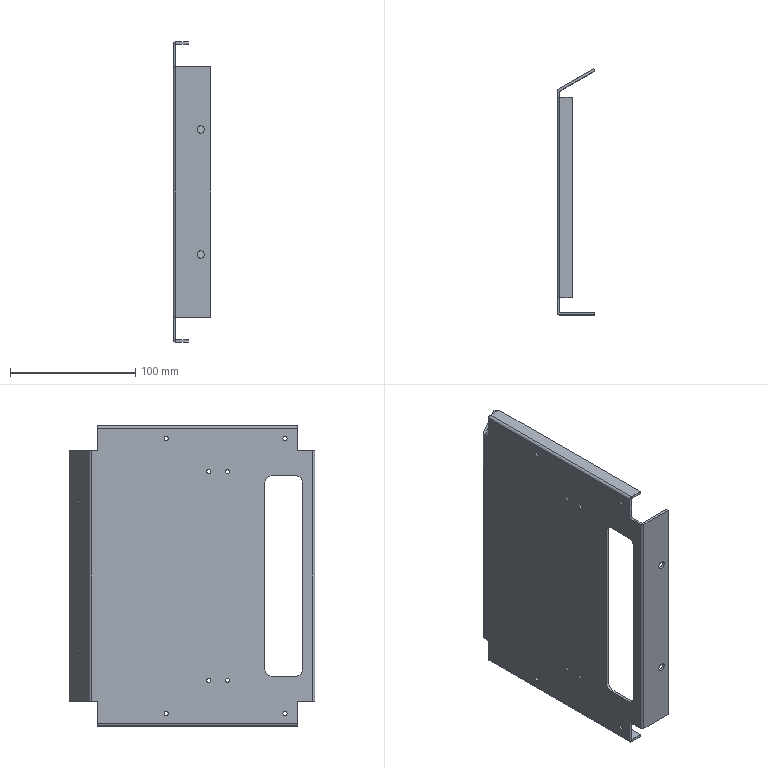Part | NX | features BREP 1 | 1 solid | 66 faces | box 30.012 x 196.75 x 240 mm | volume 105008 mm3 | plane 34 | cylinder 32 | commonest cylinder face diameters 3.3 x20 4 x4 6 x4 10 x4